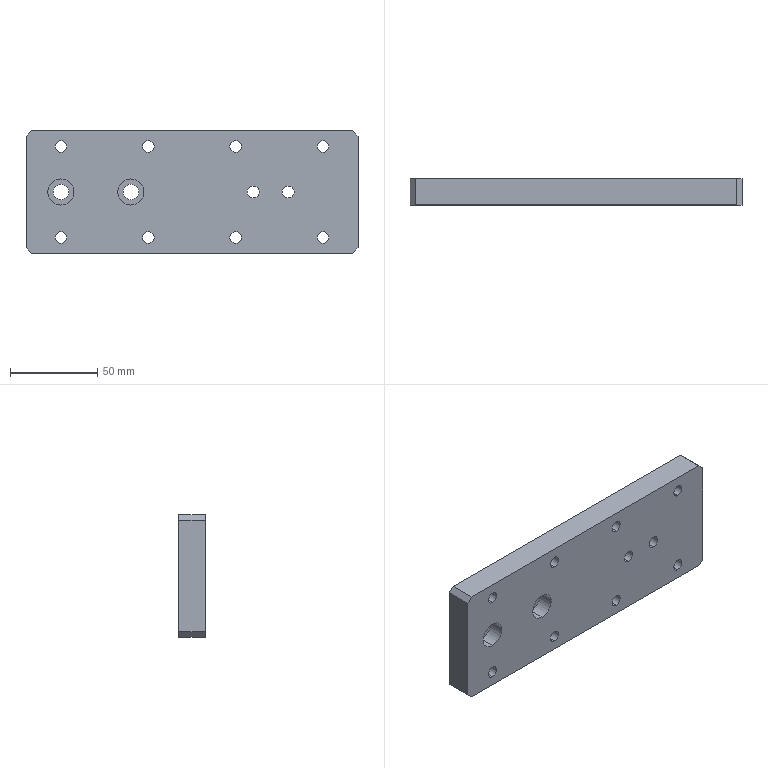Part | SolidWorks | features HoleWzd 4, Chamfer 1, Extrusion 1 | 1 solid | 64 faces | box 190 x 15 x 70 mm | volume 186782 mm3 | cylinder 44 | plane 20 | commonest cylinder face diameters 6.6 x16 11 x16 6.8 x4 9 x4 15 x4